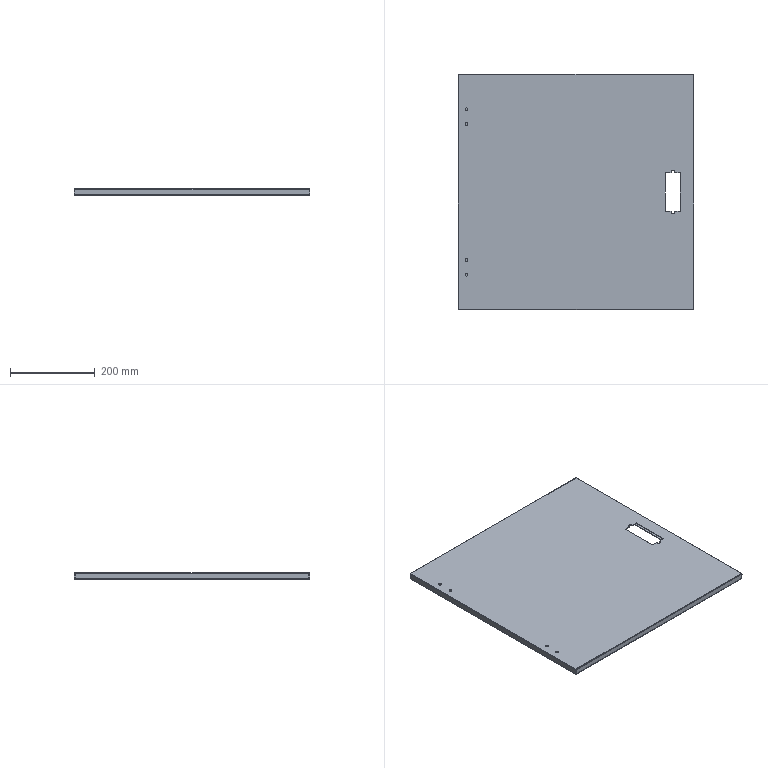Part | STEP file | Left door panel sheet metal_PN_0010 | 1 solid | 90 faces | box 558 x 557 x 15 mm | volume 577988 mm3 | plane 48 | cylinder 26 | spline 16 | commonest cylinder face diameters 0.2 x8 3.2 x8 6.5 x8 8 x2